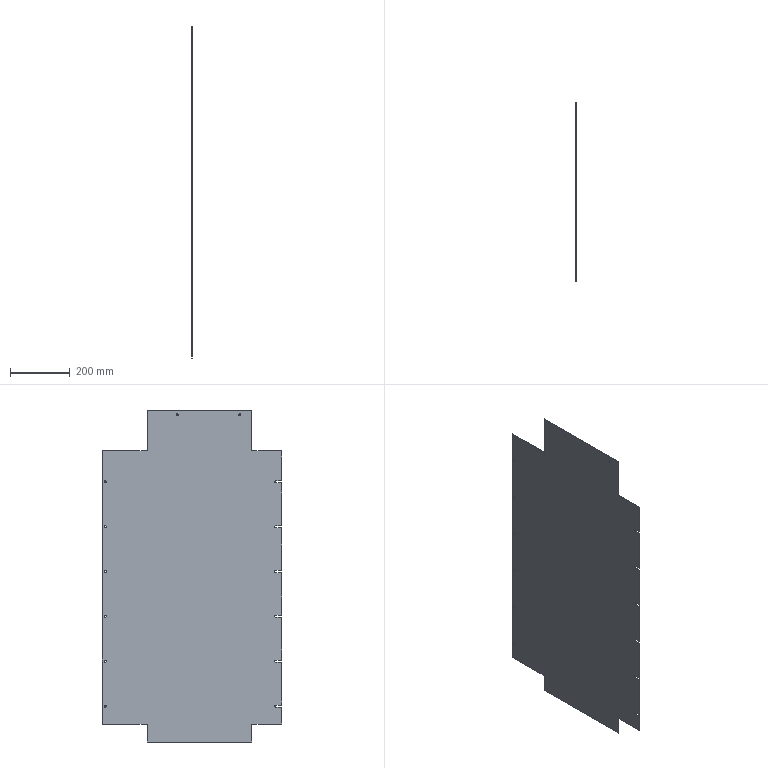Part | NX | 1 solid | 54 faces | box 2 x 600 x 1110 mm | volume 1231223 mm3 | plane 32 | cylinder 22 | commonest cylinder face diameters 7 x22